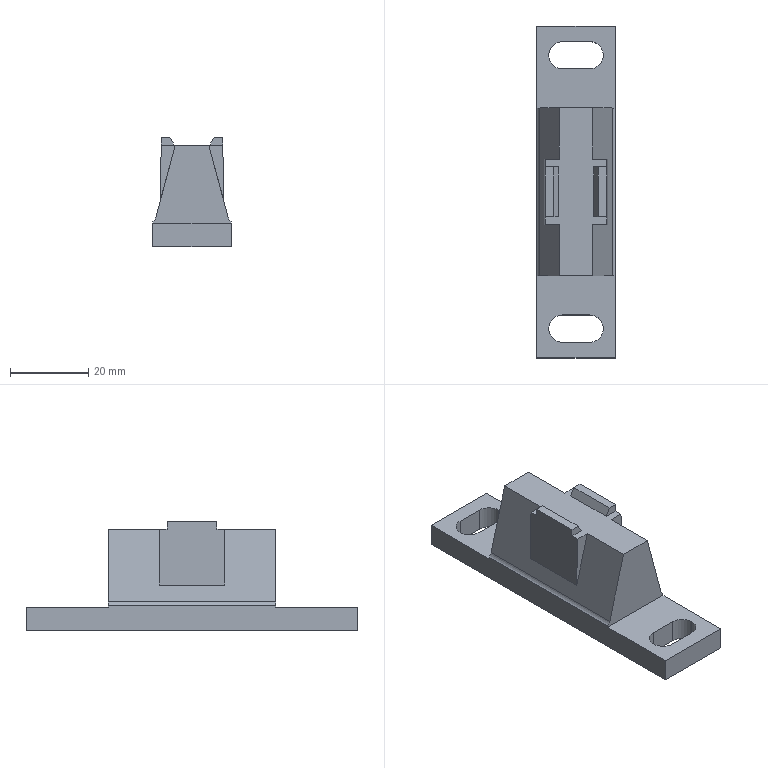Part | SolidWorks | features BaseBody 1 | 1 solid | 38 faces | box 20 x 85 x 28 mm | volume 22186 mm3 | plane 30 | cylinder 8 | commonest cylinder face diameters 7 x6 4 x2
STEP:
#1=CARTESIAN_POINT('',(7.,-35.,-41.));
#2=VERTEX_POINT('',#1);
#3=CARTESIAN_POINT('',(3.5,-31.5,-41.));
#4=VERTEX_POINT('',#3);
#5=CARTESIAN_POINT('',(3.5,-35.,-41.));
#6=DIRECTION('',(0.,0.,1.));
#7=DIRECTION('',(0.,-1.,0.));
#8=AXIS2_PLACEMENT_3D('',#5,#6,#7);
#9=CIRCLE('',#8,3.5);
#10=EDGE_CURVE('',#2,#4,#9,.T.);
#11=ORIENTED_EDGE('',*,*,#10,.F.);
#12=CARTESIAN_POINT('',(7.,-35.,-35.));
#13=VERTEX_POINT('',#12);
#14=CARTESIAN_POINT('',(7.,-35.,-41.));
#15=DIRECTION('',(0.,0.,1.));
#16=VECTOR('',#15,1000.);
#17=LINE('',#14,#16);
#18=EDGE_CURVE('',#2,#13,#17,.T.);
#19=ORIENTED_EDGE('',*,*,#18,.T.);
#20=CARTESIAN_POINT('',(3.5,-31.5,-35.));
#21=VERTEX_POINT('',#20);
#22=CARTESIAN_POINT('',(3.5,-35.,-35.));
#23=DIRECTION('',(0.,0.,1.));
#24=DIRECTION('',(0.,-1.,0.));
#25=AXIS2_PLACEMENT_3D('',#22,#23,#24);
#26=CIRCLE('',#25,3.5);
#27=EDGE_CURVE('',#13,#21,#26,.T.);
#28=ORIENTED_EDGE('',*,*,#27,.T.);
#29=CARTESIAN_POINT('',(3.5,-31.5,-41.));
#30=DIRECTION('',(0.,0.,1.));
#31=VECTOR('',#30,1000.);
#32=LINE('',#29,#31);
#33=EDGE_CURVE('',#4,#21,#32,.T.);
#34=ORIENTED_EDGE('',*,*,#33,.F.);
#35=EDGE_LOOP('',(#11,#19,#28,#34));
#36=FACE_OUTER_BOUND('',#35,.T.);
#37=CARTESIAN_POINT('',(3.5,-35.,-41.));
#38=DIRECTION('',(0.,0.,1.));
#39=DIRECTION('',(1.,0.,0.));
#40=AXIS2_PLACEMENT_3D('',#37,#38,#39);
#41=CYLINDRICAL_SURFACE('',#40,3.5);
#42=ADVANCED_FACE('',(#36),#41,.F.);
#43=CARTESIAN_POINT('',(7.,35.,-41.));
#44=VERTEX_POINT('',#43);
#45=CARTESIAN_POINT('',(3.5,38.5,-41.));
#46=VERTEX_POINT('',#45);
#47=CARTESIAN_POINT('',(3.5,35.,-41.));
#48=DIRECTION('',(0.,0.,1.));
#49=DIRECTION('',(0.,-1.,0.));
#50=AXIS2_PLACEMENT_3D('',#47,#48,#49);
#51=CIRCLE('',#50,3.5);
#52=EDGE_CURVE('',#44,#46,#51,.T.);
#53=ORIENTED_EDGE('',*,*,#52,.F.);
#54=CARTESIAN_POINT('',(7.,35.,-35.));
#55=VERTEX_POINT('',#54);
#56=CARTESIAN_POINT('',(7.,35.,-41.));
#57=DIRECTION('',(0.,0.,1.));
#58=VECTOR('',#57,1000.);
#59=LINE('',#56,#58);
#60=EDGE_CURVE('',#44,#55,#59,.T.);
#61=ORIENTED_EDGE('',*,*,#60,.T.);
#62=CARTESIAN_POINT('',(3.5,38.5,-35.));
#63=VERTEX_POINT('',#62);
#64=CARTESIAN_POINT('',(3.5,35.,-35.));
#65=DIRECTION('',(0.,0.,1.));
#66=DIRECTION('',(0.,-1.,0.));
#67=AXIS2_PLACEMENT_3D('',#64,#65,#66);
#68=CIRCLE('',#67,3.5);
#69=EDGE_CURVE('',#55,#63,#68,.T.);
#70=ORIENTED_EDGE('',*,*,#69,.T.);
#71=CARTESIAN_POINT('',(3.5,38.5,-41.));
#72=DIRECTION('',(0.,0.,1.));
#73=VECTOR('',#72,1000.);
#74=LINE('',#71,#73);
#75=EDGE_CURVE('',#46,#63,#74,.T.);
#76=ORIENTED_EDGE('',*,*,#75,.F.);
#77=EDGE_LOOP('',(#53,#61,#70,#76));
#78=FACE_OUTER_BOUND('',#77,.T.);
#79=CARTESIAN_POINT('',(3.5,35.,-41.));
#80=DIRECTION('',(0.,0.,1.));
#81=DIRECTION('',(1.,0.,0.));
#82=AXIS2_PLACEMENT_3D('',#79,#80,#81);
#83=CYLINDRICAL_SURFACE('',#82,3.5);
#84=ADVANCED_FACE('',(#78),#83,.F.);
#85=CARTESIAN_POINT('',(5.655,-6.4,-13.));
#86=VERTEX_POINT('',#85);
#87=CARTESIAN_POINT('',(4.5,-6.4,-15.));
#88=VERTEX_POINT('',#87);
#89=CARTESIAN_POINT('',(5.655,-6.4,-13.));
#90=DIRECTION('',(-0.5,0.,-0.866));
#91=VECTOR('',#90,1000.);
#92=LINE('',#89,#91);
#93=EDGE_CURVE('',#86,#88,#92,.T.);
#94=ORIENTED_EDGE('',*,*,#93,.F.);
#95=CARTESIAN_POINT('',(5.655,6.4,-13.));
#96=VERTEX_POINT('',#95);
#97=CARTESIAN_POINT('',(5.655,6.4,-13.));
#98=DIRECTION('',(0.,-1.,0.));
#99=VECTOR('',#98,1000.);
#100=LINE('',#97,#99);
#101=EDGE_CURVE('',#96,#86,#100,.T.);
#102=ORIENTED_EDGE('',*,*,#101,.F.);
#103=CARTESIAN_POINT('',(4.5,6.4,-15.));
#104=VERTEX_POINT('',#103);
#105=CARTESIAN_POINT('',(4.5,6.4,-15.));
#106=DIRECTION('',(0.5,0.,0.866));
#107=VECTOR('',#106,1000.);
#108=LINE('',#105,#107);
#109=EDGE_CURVE('',#104,#96,#108,.T.);
#110=ORIENTED_EDGE('',*,*,#109,.F.);
#111=CARTESIAN_POINT('',(4.5,6.4,-15.));
#112=DIRECTION('',(0.,-1.,0.));
#113=VECTOR('',#112,1000.);
#114=LINE('',#111,#113);
#115=EDGE_CURVE('',#104,#88,#114,.T.);
#116=ORIENTED_EDGE('',*,*,#115,.T.);
#117=EDGE_LOOP('',(#94,#102,#110,#116));
#118=FACE_OUTER_BOUND('',#117,.T.);
#119=CARTESIAN_POINT('',(4.5,8.4,-15.));
#120=DIRECTION('',(0.866,0.,-0.5));
#121=DIRECTION('',(-0.5,0.,-0.866));
#122=AXIS2_PLACEMENT_3D('',#119,#120,#121);
#123=PLANE('',#122);
#124=ADVANCED_FACE('',(#118),#123,.F.);
#125=ORIENTED_EDGE('',*,*,#93,.T.);
#126=CARTESIAN_POINT('',(7.885,-6.4,-15.));
#127=VERTEX_POINT('',#126);
#128=CARTESIAN_POINT('',(7.885,-6.4,-15.));
#129=DIRECTION('',(-1.,0.,0.));
#130=VECTOR('',#129,1000.);
#131=LINE('',#128,#130);
#132=EDGE_CURVE('',#127,#88,#131,.T.);
#133=ORIENTED_EDGE('',*,*,#132,.F.);
#134=CARTESIAN_POINT('',(7.85,-6.4,-13.));
#135=VERTEX_POINT('',#134);
#136=CARTESIAN_POINT('',(7.885,-6.4,-15.));
#137=DIRECTION('',(-0.01745,0.,0.9998));
#138=VECTOR('',#137,1000.);
#139=LINE('',#136,#138);
#140=EDGE_CURVE('',#127,#135,#139,.T.);
#141=ORIENTED_EDGE('',*,*,#140,.T.);
#142=CARTESIAN_POINT('',(7.85,-6.4,-13.));
#143=DIRECTION('',(-1.,0.,0.));
#144=VECTOR('',#143,1000.);
#145=LINE('',#142,#144);
#146=EDGE_CURVE('',#135,#86,#145,.T.);
#147=ORIENTED_EDGE('',*,*,#146,.T.);
#148=EDGE_LOOP('',(#125,#133,#141,#147));
#149=FACE_OUTER_BOUND('',#148,.T.);
#150=CARTESIAN_POINT('',(10.,-6.4,-15.));
#151=DIRECTION('',(0.,-1.,0.));
#152=DIRECTION('',(0.,0.,-1.));
#153=AXIS2_PLACEMENT_3D('',#150,#151,#152);
#154=PLANE('',#153);
#155=ADVANCED_FACE('',(#149),#154,.T.);
#156=ORIENTED_EDGE('',*,*,#146,.F.);
#157=CARTESIAN_POINT('',(7.85,6.4,-13.));
#158=VERTEX_POINT('',#157);
#159=CARTESIAN_POINT('',(7.85,6.4,-13.));
#160=DIRECTION('',(0.,-1.,0.));
#161=VECTOR('',#160,1000.);
#162=LINE('',#159,#161);
#163=EDGE_CURVE('',#158,#135,#162,.T.);
#164=ORIENTED_EDGE('',*,*,#163,.F.);
#165=CARTESIAN_POINT('',(5.655,6.4,-13.));
#166=DIRECTION('',(1.,0.,0.));
#167=VECTOR('',#166,1000.);
#168=LINE('',#165,#167);
#169=EDGE_CURVE('',#96,#158,#168,.T.);
#170=ORIENTED_EDGE('',*,*,#169,.F.);
#171=ORIENTED_EDGE('',*,*,#101,.T.);
#172=EDGE_LOOP('',(#156,#164,#170,#171));
#173=FACE_OUTER_BOUND('',#172,.T.);
#174=CARTESIAN_POINT('',(5.655,8.4,-13.));
#175=DIRECTION('',(0.,0.,-1.));
#176=DIRECTION('',(-1.,0.,0.));
#177=AXIS2_PLACEMENT_3D('',#174,#175,#176);
#178=PLANE('',#177);
#179=ADVANCED_FACE('',(#173),#178,.F.);
#180=ORIENTED_EDGE('',*,*,#109,.T.);
#181=ORIENTED_EDGE('',*,*,#169,.T.);
#182=CARTESIAN_POINT('',(7.885,6.4,-15.));
#183=VERTEX_POINT('',#182);
#184=CARTESIAN_POINT('',(7.85,6.4,-13.));
#185=DIRECTION('',(0.01745,0.,-0.9998));
#186=VECTOR('',#185,1000.);
#187=LINE('',#184,#186);
#188=EDGE_CURVE('',#158,#183,#187,.T.);
#189=ORIENTED_EDGE('',*,*,#188,.T.);
#190=CARTESIAN_POINT('',(7.885,6.4,-15.));
#191=DIRECTION('',(-1.,0.,0.));
#192=VECTOR('',#191,1000.);
#193=LINE('',#190,#192);
#194=EDGE_CURVE('',#183,#104,#193,.T.);
#195=ORIENTED_EDGE('',*,*,#194,.T.);
#196=EDGE_LOOP('',(#180,#181,#189,#195));
#197=FACE_OUTER_BOUND('',#196,.T.);
#198=CARTESIAN_POINT('',(10.,6.4,-12.));
#199=DIRECTION('',(0.,1.,0.));
#200=DIRECTION('',(0.,0.,1.));
#201=AXIS2_PLACEMENT_3D('',#198,#199,#200);
#202=PLANE('',#201);
#203=ADVANCED_FACE('',(#197),#202,.T.);
#204=CARTESIAN_POINT('',(4.3,8.4,-15.));
#205=VERTEX_POINT('',#204);
#206=CARTESIAN_POINT('',(7.885,8.4,-15.));
#207=VERTEX_POINT('',#206);
#208=CARTESIAN_POINT('',(4.3,8.4,-15.));
#209=DIRECTION('',(1.,0.,0.));
#210=VECTOR('',#209,1000.);
#211=LINE('',#208,#210);
#212=EDGE_CURVE('',#205,#207,#211,.T.);
#213=ORIENTED_EDGE('',*,*,#212,.F.);
#214=CARTESIAN_POINT('',(4.3,21.5,-15.));
#215=VERTEX_POINT('',#214);
#216=CARTESIAN_POINT('',(4.3,21.5,-15.));
#217=DIRECTION('',(0.,-1.,0.));
#218=VECTOR('',#217,1000.);
#219=LINE('',#216,#218);
#220=EDGE_CURVE('',#215,#205,#219,.T.);
#221=ORIENTED_EDGE('',*,*,#220,.F.);
#222=CARTESIAN_POINT('',(-4.3,21.5,-15.));
#223=VERTEX_POINT('',#222);
#224=CARTESIAN_POINT('',(-4.3,21.5,-15.));
#225=DIRECTION('',(1.,0.,0.));
#226=VECTOR('',#225,1000.);
#227=LINE('',#224,#226);
#228=EDGE_CURVE('',#223,#215,#227,.T.);
#229=ORIENTED_EDGE('',*,*,#228,.F.);
#230=CARTESIAN_POINT('',(-4.3,8.4,-15.));
#231=VERTEX_POINT('',#230);
#232=CARTESIAN_POINT('',(-4.3,21.5,-15.));
#233=DIRECTION('',(0.,-1.,0.));
#234=VECTOR('',#233,1000.);
#235=LINE('',#232,#234);
#236=EDGE_CURVE('',#223,#231,#235,.T.);
#237=ORIENTED_EDGE('',*,*,#236,.T.);
#238=CARTESIAN_POINT('',(-7.885,8.4,-15.));
#239=VERTEX_POINT('',#238);
#240=CARTESIAN_POINT('',(-7.885,8.4,-15.));
#241=DIRECTION('',(1.,0.,0.));
#242=VECTOR('',#241,1000.);
#243=LINE('',#240,#242);
#244=EDGE_CURVE('',#239,#231,#243,.T.);
#245=ORIENTED_EDGE('',*,*,#244,.F.);
#246=CARTESIAN_POINT('',(-7.885,6.4,-15.));
#247=VERTEX_POINT('',#246);
#248=CARTESIAN_POINT('',(-7.885,8.4,-15.));
#249=DIRECTION('',(0.,-1.,0.));
#250=VECTOR('',#249,1000.);
#251=LINE('',#248,#250);
#252=EDGE_CURVE('',#239,#247,#251,.T.);
#253=ORIENTED_EDGE('',*,*,#252,.T.);
#254=CARTESIAN_POINT('',(-4.5,6.4,-15.));
#255=VERTEX_POINT('',#254);
#256=CARTESIAN_POINT('',(-4.5,6.4,-15.));
#257=DIRECTION('',(-1.,0.,0.));
#258=VECTOR('',#257,1000.);
#259=LINE('',#256,#258);
#260=EDGE_CURVE('',#255,#247,#259,.T.);
#261=ORIENTED_EDGE('',*,*,#260,.F.);
#262=CARTESIAN_POINT('',(-4.5,-6.4,-15.));
#263=VERTEX_POINT('',#262);
#264=CARTESIAN_POINT('',(-4.5,6.4,-15.));
#265=DIRECTION('',(0.,-1.,0.));
#266=VECTOR('',#265,1000.);
#267=LINE('',#264,#266);
#268=EDGE_CURVE('',#255,#263,#267,.T.);
#269=ORIENTED_EDGE('',*,*,#268,.T.);
#270=CARTESIAN_POINT('',(-7.885,-6.4,-15.));
#271=VERTEX_POINT('',#270);
#272=CARTESIAN_POINT('',(-4.5,-6.4,-15.));
#273=DIRECTION('',(-1.,0.,0.));
#274=VECTOR('',#273,1000.);
#275=LINE('',#272,#274);
#276=EDGE_CURVE('',#263,#271,#275,.T.);
#277=ORIENTED_EDGE('',*,*,#276,.T.);
#278=CARTESIAN_POINT('',(-7.885,-8.4,-15.));
#279=VERTEX_POINT('',#278);
#280=CARTESIAN_POINT('',(-7.885,-6.4,-15.));
#281=DIRECTION('',(0.,-1.,0.));
#282=VECTOR('',#281,1000.);
#283=LINE('',#280,#282);
#284=EDGE_CURVE('',#271,#279,#283,.T.);
#285=ORIENTED_EDGE('',*,*,#284,.T.);
#286=CARTESIAN_POINT('',(-4.3,-8.4,-15.));
#287=VERTEX_POINT('',#286);
#288=CARTESIAN_POINT('',(-7.885,-8.4,-15.));
#289=DIRECTION('',(1.,0.,0.));
#290=VECTOR('',#289,1000.);
#291=LINE('',#288,#290);
#292=EDGE_CURVE('',#279,#287,#291,.T.);
#293=ORIENTED_EDGE('',*,*,#292,.T.);
#294=CARTESIAN_POINT('',(-4.3,-21.5,-15.));
#295=VERTEX_POINT('',#294);
#296=CARTESIAN_POINT('',(-4.3,-8.4,-15.));
#297=DIRECTION('',(0.,-1.,0.));
#298=VECTOR('',#297,1000.);
#299=LINE('',#296,#298);
#300=EDGE_CURVE('',#287,#295,#299,.T.);
#301=ORIENTED_EDGE('',*,*,#300,.T.);
#302=CARTESIAN_POINT('',(4.3,-21.5,-15.));
#303=VERTEX_POINT('',#302);
#304=CARTESIAN_POINT('',(-4.3,-21.5,-15.));
#305=DIRECTION('',(1.,0.,0.));
#306=VECTOR('',#305,1000.);
#307=LINE('',#304,#306);
#308=EDGE_CURVE('',#295,#303,#307,.T.);
#309=ORIENTED_EDGE('',*,*,#308,.T.);
#310=CARTESIAN_POINT('',(4.3,-8.4,-15.));
#311=VERTEX_POINT('',#310);
#312=CARTESIAN_POINT('',(4.3,-8.4,-15.));
#313=DIRECTION('',(0.,-1.,0.));
#314=VECTOR('',#313,1000.);
#315=LINE('',#312,#314);
#316=EDGE_CURVE('',#311,#303,#315,.T.);
#317=ORIENTED_EDGE('',*,*,#316,.F.);
#318=CARTESIAN_POINT('',(7.885,-8.4,-15.));
#319=VERTEX_POINT('',#318);
#320=CARTESIAN_POINT('',(4.3,-8.4,-15.));
#321=DIRECTION('',(1.,0.,0.));
#322=VECTOR('',#321,1000.);
#323=LINE('',#320,#322);
#324=EDGE_CURVE('',#311,#319,#323,.T.);
#325=ORIENTED_EDGE('',*,*,#324,.T.);
#326=CARTESIAN_POINT('',(7.885,-8.4,-15.));
#327=DIRECTION('',(0.,1.,0.));
#328=VECTOR('',#327,1000.);
#329=LINE('',#326,#328);
#330=EDGE_CURVE('',#319,#127,#329,.T.);
#331=ORIENTED_EDGE('',*,*,#330,.T.);
#332=ORIENTED_EDGE('',*,*,#132,.T.);
#333=ORIENTED_EDGE('',*,*,#115,.F.);
#334=ORIENTED_EDGE('',*,*,#194,.F.);
#335=CARTESIAN_POINT('',(7.885,6.4,-15.));
#336=DIRECTION('',(0.,1.,0.));
#337=VECTOR('',#336,1000.);
#338=LINE('',#335,#337);
#339=EDGE_CURVE('',#183,#207,#338,.T.);
#340=ORIENTED_EDGE('',*,*,#339,.T.);
#341=EDGE_LOOP('',(#213,#221,#229,#237,#245,#253,#261,#269,#277,#285,#293,#301,#309,#317,#325,#331,#332,#333,#334,#340));
#342=FACE_OUTER_BOUND('',#341,.T.);
#343=CARTESIAN_POINT('',(-4.3,21.5,-15.));
#344=DIRECTION('',(0.,0.,-1.));
#345=DIRECTION('',(-1.,0.,0.));
#346=AXIS2_PLACEMENT_3D('',#343,#344,#345);
#347=PLANE('',#346);
#348=ADVANCED_FACE('',(#342),#347,.F.);
#349=ORIENTED_EDGE('',*,*,#330,.F.);
#350=CARTESIAN_POINT('',(8.135,-8.4,-29.311));
#351=VERTEX_POINT('',#350);
#352=CARTESIAN_POINT('',(7.885,-8.4,-15.));
#353=DIRECTION('',(0.01745,0.,-0.9998));
#354=VECTOR('',#353,1000.);
#355=LINE('',#352,#354);
#356=EDGE_CURVE('',#319,#351,#355,.T.);
#357=ORIENTED_EDGE('',*,*,#356,.T.);
#358=CARTESIAN_POINT('',(8.135,8.4,-29.311));
#359=VERTEX_POINT('',#358);
#360=CARTESIAN_POINT('',(8.135,-8.4,-29.311));
#361=DIRECTION('',(0.,1.,0.));
#362=VECTOR('',#361,1000.);
#363=LINE('',#360,#362);
#364=EDGE_CURVE('',#351,#359,#363,.T.);
#365=ORIENTED_EDGE('',*,*,#364,.T.);
#366=CARTESIAN_POINT('',(7.885,8.4,-15.));
#367=DIRECTION('',(0.01745,0.,-0.9998));
#368=VECTOR('',#367,1000.);
#369=LINE('',#366,#368);
#370=EDGE_CURVE('',#207,#359,#369,.T.);
#371=ORIENTED_EDGE('',*,*,#370,.F.);
#372=ORIENTED_EDGE('',*,*,#339,.F.);
#373=ORIENTED_EDGE('',*,*,#188,.F.);
#374=ORIENTED_EDGE('',*,*,#163,.T.);
#375=ORIENTED_EDGE('',*,*,#140,.F.);
#376=EDGE_LOOP('',(#349,#357,#365,#371,#372,#373,#374,#375));
#377=FACE_OUTER_BOUND('',#376,.T.);
#378=CARTESIAN_POINT('',(7.85,8.4,-13.));
#379=DIRECTION('',(-0.9998,0.,-0.01745));
#380=DIRECTION('',(-0.01745,0.,0.9998));
#381=AXIS2_PLACEMENT_3D('',#378,#379,#380);
#382=PLANE('',#381);
#383=ADVANCED_FACE('',(#377),#382,.F.);
#384=ORIENTED_EDGE('',*,*,#212,.T.);
#385=ORIENTED_EDGE('',*,*,#370,.T.);
#386=CARTESIAN_POINT('',(4.3,8.4,-15.));
#387=DIRECTION('',(0.2588,0.,-0.9659));
#388=VECTOR('',#387,1000.);
#389=LINE('',#386,#388);
#390=EDGE_CURVE('',#205,#359,#389,.T.);
#391=ORIENTED_EDGE('',*,*,#390,.F.);
#392=EDGE_LOOP('',(#384,#385,#391));
#393=FACE_OUTER_BOUND('',#392,.T.);
#394=CARTESIAN_POINT('',(0.,8.4,0.));
#395=DIRECTION('',(0.,1.,0.));
#396=DIRECTION('',(0.,0.,1.));
#397=AXIS2_PLACEMENT_3D('',#394,#395,#396);
#398=PLANE('',#397);
#399=ADVANCED_FACE('',(#393),#398,.T.);
#400=ORIENTED_EDGE('',*,*,#220,.T.);
#401=ORIENTED_EDGE('',*,*,#390,.T.);
#402=ORIENTED_EDGE('',*,*,#364,.F.);
#403=CARTESIAN_POINT('',(4.3,-8.4,-15.));
#404=DIRECTION('',(0.2588,0.,-0.9659));
#405=VECTOR('',#404,1000.);
#406=LINE('',#403,#405);
#407=EDGE_CURVE('',#311,#351,#406,.T.);
#408=ORIENTED_EDGE('',*,*,#407,.F.);
#409=ORIENTED_EDGE('',*,*,#316,.T.);
#410=CARTESIAN_POINT('',(9.262,-21.5,-33.518));
#411=VERTEX_POINT('',#410);
#412=CARTESIAN_POINT('',(4.3,-21.5,-15.));
#413=DIRECTION('',(0.2588,0.,-0.9659));
#414=VECTOR('',#413,1000.);
#415=LINE('',#412,#414);
#416=EDGE_CURVE('',#303,#411,#415,.T.);
#417=ORIENTED_EDGE('',*,*,#416,.T.);
#418=CARTESIAN_POINT('',(9.262,21.5,-33.518));
#419=VERTEX_POINT('',#418);
#420=CARTESIAN_POINT('',(9.262,21.5,-33.518));
#421=DIRECTION('',(0.,-1.,0.));
#422=VECTOR('',#421,1000.);
#423=LINE('',#420,#422);
#424=EDGE_CURVE('',#419,#411,#423,.T.);
#425=ORIENTED_EDGE('',*,*,#424,.F.);
#426=CARTESIAN_POINT('',(4.3,21.5,-15.));
#427=DIRECTION('',(0.2588,0.,-0.9659));
#428=VECTOR('',#427,1000.);
#429=LINE('',#426,#428);
#430=EDGE_CURVE('',#215,#419,#429,.T.);
#431=ORIENTED_EDGE('',*,*,#430,.F.);
#432=EDGE_LOOP('',(#400,#401,#402,#408,#409,#417,#425,#431));
#433=FACE_OUTER_BOUND('',#432,.T.);
#434=CARTESIAN_POINT('',(4.3,21.5,-15.));
#435=DIRECTION('',(-0.9659,0.,-0.2588));
#436=DIRECTION('',(-0.2588,0.,0.9659));
#437=AXIS2_PLACEMENT_3D('',#434,#435,#436);
#438=PLANE('',#437);
#439=ADVANCED_FACE('',(#433),#438,.F.);
#440=CARTESIAN_POINT('',(-10.,21.5,-35.));
#441=VERTEX_POINT('',#440);
#442=CARTESIAN_POINT('',(-10.,21.5,-34.605));
#443=VERTEX_POINT('',#442);
#444=CARTESIAN_POINT('',(-10.,21.5,-35.));
#445=DIRECTION('',(0.,0.,1.));
#446=VECTOR('',#445,1000.);
#447=LINE('',#444,#446);
#448=EDGE_CURVE('',#441,#443,#447,.T.);
#449=ORIENTED_EDGE('',*,*,#448,.T.);
#450=CARTESIAN_POINT('',(-9.262,21.5,-33.518));
#451=VERTEX_POINT('',#450);
#452=CARTESIAN_POINT('',(-11.194,21.5,-33.));
#453=DIRECTION('',(0.,1.,0.));
#454=DIRECTION('',(0.9659,0.,-0.2588));
#455=AXIS2_PLACEMENT_3D('',#452,#453,#454);
#456=CIRCLE('',#455,2.);
#457=EDGE_CURVE('',#451,#443,#456,.T.);
#458=ORIENTED_EDGE('',*,*,#457,.F.);
#459=CARTESIAN_POINT('',(-9.262,21.5,-33.518));
#460=DIRECTION('',(0.2588,0.,0.9659));
#461=VECTOR('',#460,1000.);
#462=LINE('',#459,#461);
#463=EDGE_CURVE('',#451,#223,#462,.T.);
#464=ORIENTED_EDGE('',*,*,#463,.T.);
#465=ORIENTED_EDGE('',*,*,#228,.T.);
#466=ORIENTED_EDGE('',*,*,#430,.T.);
#467=CARTESIAN_POINT('',(10.,21.5,-34.605));
#468=VERTEX_POINT('',#467);
#469=CARTESIAN_POINT('',(11.194,21.5,-33.));
#470=DIRECTION('',(0.,1.,0.));
#471=DIRECTION('',(-0.5968,0.,-0.8024));
#472=AXIS2_PLACEMENT_3D('',#469,#470,#471);
#473=CIRCLE('',#472,2.);
#474=EDGE_CURVE('',#468,#419,#473,.T.);
#475=ORIENTED_EDGE('',*,*,#474,.F.);
#476=CARTESIAN_POINT('',(10.,21.5,-35.));
#477=VERTEX_POINT('',#476);
#478=CARTESIAN_POINT('',(10.,21.5,-34.605));
#479=DIRECTION('',(0.,0.,-1.));
#480=VECTOR('',#479,1000.);
#481=LINE('',#478,#480);
#482=EDGE_CURVE('',#468,#477,#481,.T.);
#483=ORIENTED_EDGE('',*,*,#482,.T.);
#484=CARTESIAN_POINT('',(10.,21.5,-35.));
#485=DIRECTION('',(-1.,0.,0.));
#486=VECTOR('',#485,1000.);
#487=LINE('',#484,#486);
#488=EDGE_CURVE('',#477,#441,#487,.T.);
#489=ORIENTED_EDGE('',*,*,#488,.T.);
#490=EDGE_LOOP('',(#449,#458,#464,#465,#466,#475,#483,#489));
#491=FACE_OUTER_BOUND('',#490,.T.);
#492=CARTESIAN_POINT('',(-11.194,21.5,-33.));
#493=DIRECTION('',(0.,1.,0.));
#494=DIRECTION('',(0.,0.,1.));
#495=AXIS2_PLACEMENT_3D('',#492,#493,#494);
#496=PLANE('',#495);
#497=ADVANCED_FACE('',(#491),#496,.T.);
#498=CARTESIAN_POINT('',(-8.135,8.4,-29.311));
#499=VERTEX_POINT('',#498);
#500=CARTESIAN_POINT('',(-8.135,-8.4,-29.311));
#501=VERTEX_POINT('',#500);
#502=CARTESIAN_POINT('',(-8.135,8.4,-29.311));
#503=DIRECTION('',(0.,-1.,0.));
#504=VECTOR('',#503,1000.);
#505=LINE('',#502,#504);
#506=EDGE_CURVE('',#499,#501,#505,.T.);
#507=ORIENTED_EDGE('',*,*,#506,.F.);
#508=CARTESIAN_POINT('',(-8.135,8.4,-29.311));
#509=DIRECTION('',(0.2588,0.,0.9659));
#510=VECTOR('',#509,1000.);
#511=LINE('',#508,#510);
#512=EDGE_CURVE('',#499,#231,#511,.T.);
#513=ORIENTED_EDGE('',*,*,#512,.T.);
#514=ORIENTED_EDGE('',*,*,#236,.F.);
#515=ORIENTED_EDGE('',*,*,#463,.F.);
#516=CARTESIAN_POINT('',(-9.262,-21.5,-33.518));
#517=VERTEX_POINT('',#516);
#518=CARTESIAN_POINT('',(-9.262,21.5,-33.518));
#519=DIRECTION('',(0.,-1.,0.));
#520=VECTOR('',#519,1000.);
#521=LINE('',#518,#520);
#522=EDGE_CURVE('',#451,#517,#521,.T.);
#523=ORIENTED_EDGE('',*,*,#522,.T.);
#524=CARTESIAN_POINT('',(-9.262,-21.5,-33.518));
#525=DIRECTION('',(0.2588,0.,0.9659));
#526=VECTOR('',#525,1000.);
#527=LINE('',#524,#526);
#528=EDGE_CURVE('',#517,#295,#527,.T.);
#529=ORIENTED_EDGE('',*,*,#528,.T.);
#530=ORIENTED_EDGE('',*,*,#300,.F.);
#531=CARTESIAN_POINT('',(-8.135,-8.4,-29.311));
#532=DIRECTION('',(0.2588,0.,0.9659));
#533=VECTOR('',#532,1000.);
#534=LINE('',#531,#533);
#535=EDGE_CURVE('',#501,#287,#534,.T.);
#536=ORIENTED_EDGE('',*,*,#535,.F.);
#537=EDGE_LOOP('',(#507,#513,#514,#515,#523,#529,#530,#536));
#538=FACE_OUTER_BOUND('',#537,.T.);
#539=CARTESIAN_POINT('',(-9.262,21.5,-33.518));
#540=DIRECTION('',(0.9659,0.,-0.2588));
#541=DIRECTION('',(-0.2588,0.,-0.9659));
#542=AXIS2_PLACEMENT_3D('',#539,#540,#541);
#543=PLANE('',#542);
#544=ADVANCED_FACE('',(#538),#543,.F.);
#545=CARTESIAN_POINT('',(-8.135,8.4,-29.311));
#546=DIRECTION('',(0.01745,0.,0.9998));
#547=VECTOR('',#546,1000.);
#548=LINE('',#545,#547);
#549=EDGE_CURVE('',#499,#239,#548,.T.);
#550=ORIENTED_EDGE('',*,*,#549,.T.);
#551=ORIENTED_EDGE('',*,*,#244,.T.);
#552=ORIENTED_EDGE('',*,*,#512,.F.);
#553=EDGE_LOOP('',(#550,#551,#552));
#554=FACE_OUTER_BOUND('',#553,.T.);
#555=CARTESIAN_POINT('',(0.,8.4,0.));
#556=DIRECTION('',(0.,1.,0.));
#557=DIRECTION('',(0.,0.,1.));
#558=AXIS2_PLACEMENT_3D('',#555,#556,#557);
#559=PLANE('',#558);
#560=ADVANCED_FACE('',(#554),#559,.T.);
#561=ORIENTED_EDGE('',*,*,#284,.F.);
#562=CARTESIAN_POINT('',(-7.85,-6.4,-13.));
#563=VERTEX_POINT('',#562);
#564=CARTESIAN_POINT('',(-7.85,-6.4,-13.));
#565=DIRECTION('',(-0.01745,0.,-0.9998));
#566=VECTOR('',#565,1000.);
#567=LINE('',#564,#566);
#568=EDGE_CURVE('',#563,#271,#567,.T.);
#569=ORIENTED_EDGE('',*,*,#568,.F.);
#570=CARTESIAN_POINT('',(-7.85,6.4,-13.));
#571=VERTEX_POINT('',#570);
#572=CARTESIAN_POINT('',(-7.85,6.4,-13.));
#573=DIRECTION('',(0.,-1.,0.));
#574=VECTOR('',#573,1000.);
#575=LINE('',#572,#574);
#576=EDGE_CURVE('',#571,#563,#575,.T.);
#577=ORIENTED_EDGE('',*,*,#576,.F.);
#578=CARTESIAN_POINT('',(-7.885,6.4,-15.));
#579=DIRECTION('',(0.01745,0.,0.9998));
#580=VECTOR('',#579,1000.);
#581=LINE('',#578,#580);
#582=EDGE_CURVE('',#247,#571,#581,.T.);
#583=ORIENTED_EDGE('',*,*,#582,.F.);
#584=ORIENTED_EDGE('',*,*,#252,.F.);
#585=ORIENTED_EDGE('',*,*,#549,.F.);
#586=ORIENTED_EDGE('',*,*,#506,.T.);
#587=CARTESIAN_POINT('',(-8.135,-8.4,-29.311));
#588=DIRECTION('',(0.01745,0.,0.9998));
#589=VECTOR('',#588,1000.);
#590=LINE('',#587,#589);
#591=EDGE_CURVE('',#501,#279,#590,.T.);
#592=ORIENTED_EDGE('',*,*,#591,.T.);
#593=EDGE_LOOP('',(#561,#569,#577,#583,#584,#585,#586,#592));
#594=FACE_OUTER_BOUND('',#593,.T.);
#595=CARTESIAN_POINT('',(-8.234,8.4,-35.));
#596=DIRECTION('',(0.9998,0.,-0.01745));
#597=DIRECTION('',(-0.01745,0.,-0.9998));
#598=AXIS2_PLACEMENT_3D('',#595,#596,#597);
#599=PLANE('',#598);
#600=ADVANCED_FACE('',(#594),#599,.F.);
#601=ORIENTED_EDGE('',*,*,#582,.T.);
#602=CARTESIAN_POINT('',(-5.655,6.4,-13.));
#603=VERTEX_POINT('',#602);
#604=CARTESIAN_POINT('',(-7.85,6.4,-13.));
#605=DIRECTION('',(1.,0.,0.));
#606=VECTOR('',#605,1000.);
#607=LINE('',#604,#606);
#608=EDGE_CURVE('',#571,#603,#607,.T.);
#609=ORIENTED_EDGE('',*,*,#608,.T.);
#610=CARTESIAN_POINT('',(-5.655,6.4,-13.));
#611=DIRECTION('',(0.5,0.,-0.866));
#612=VECTOR('',#611,1000.);
#613=LINE('',#610,#612);
#614=EDGE_CURVE('',#603,#255,#613,.T.);
#615=ORIENTED_EDGE('',*,*,#614,.T.);
#616=ORIENTED_EDGE('',*,*,#260,.T.);
#617=EDGE_LOOP('',(#601,#609,#615,#616));
#618=FACE_OUTER_BOUND('',#617,.T.);
#619=CARTESIAN_POINT('',(10.,6.4,-12.));
#620=DIRECTION('',(0.,1.,0.));
#621=DIRECTION('',(0.,0.,1.));
#622=AXIS2_PLACEMENT_3D('',#619,#620,#621);
#623=PLANE('',#622);
#624=ADVANCED_FACE('',(#618),#623,.T.);
#625=CARTESIAN_POINT('',(-5.655,-6.4,-13.));
#626=VERTEX_POINT('',#625);
#627=CARTESIAN_POINT('',(-4.5,-6.4,-15.));
#628=DIRECTION('',(-0.5,0.,0.866));
#629=VECTOR('',#628,1000.);
#630=LINE('',#627,#629);
#631=EDGE_CURVE('',#263,#626,#630,.T.);
#632=ORIENTED_EDGE('',*,*,#631,.F.);
#633=ORIENTED_EDGE('',*,*,#268,.F.);
#634=ORIENTED_EDGE('',*,*,#614,.F.);
#635=CARTESIAN_POINT('',(-5.655,6.4,-13.));
#636=DIRECTION('',(0.,-1.,0.));
#637=VECTOR('',#636,1000.);
#638=LINE('',#635,#637);
#639=EDGE_CURVE('',#603,#626,#638,.T.);
#640=ORIENTED_EDGE('',*,*,#639,.T.);
#641=EDGE_LOOP('',(#632,#633,#634,#640));
#642=FACE_OUTER_BOUND('',#641,.T.);
#643=CARTESIAN_POINT('',(-5.655,8.4,-13.));
#644=DIRECTION('',(-0.866,0.,-0.5));
#645=DIRECTION('',(-0.5,0.,0.866));
#646=AXIS2_PLACEMENT_3D('',#643,#644,#645);
#647=PLANE('',#646);
#648=ADVANCED_FACE('',(#642),#647,.F.);
#649=ORIENTED_EDGE('',*,*,#568,.T.);
#650=ORIENTED_EDGE('',*,*,#276,.F.);
#651=ORIENTED_EDGE('',*,*,#631,.T.);
#652=CARTESIAN_POINT('',(-5.655,-6.4,-13.));
#653=DIRECTION('',(-1.,0.,0.));
#654=VECTOR('',#653,1000.);
#655=LINE('',#652,#654);
#656=EDGE_CURVE('',#626,#563,#655,.T.);
#657=ORIENTED_EDGE('',*,*,#656,.T.);
#658=EDGE_LOOP('',(#649,#650,#651,#657));
#659=FACE_OUTER_BOUND('',#658,.T.);
#660=CARTESIAN_POINT('',(10.,-6.4,-15.));
#661=DIRECTION('',(0.,-1.,0.));
#662=DIRECTION('',(0.,0.,-1.));
#663=AXIS2_PLACEMENT_3D('',#660,#661,#662);
#664=PLANE('',#663);
#665=ADVANCED_FACE('',(#659),#664,.T.);
#666=ORIENTED_EDGE('',*,*,#292,.F.);
#667=ORIENTED_EDGE('',*,*,#591,.F.);
#668=ORIENTED_EDGE('',*,*,#535,.T.);
#669=EDGE_LOOP('',(#666,#667,#668));
#670=FACE_OUTER_BOUND('',#669,.T.);
#671=CARTESIAN_POINT('',(0.,-8.4,0.));
#672=DIRECTION('',(0.,1.,0.));
#673=DIRECTION('',(0.,0.,1.));
#674=AXIS2_PLACEMENT_3D('',#671,#672,#673);
#675=PLANE('',#674);
#676=ADVANCED_FACE('',(#670),#675,.F.);
#677=CARTESIAN_POINT('',(-10.,-21.5,-35.));
#678=VERTEX_POINT('',#677);
#679=CARTESIAN_POINT('',(-10.,-21.5,-34.605));
#680=VERTEX_POINT('',#679);
#681=CARTESIAN_POINT('',(-10.,-21.5,-35.));
#682=DIRECTION('',(0.,0.,1.));
#683=VECTOR('',#682,1000.);
#684=LINE('',#681,#683);
#685=EDGE_CURVE('',#678,#680,#684,.T.);
#686=ORIENTED_EDGE('',*,*,#685,.F.);
#687=CARTESIAN_POINT('',(10.,-21.5,-35.));
#688=VERTEX_POINT('',#687);
#689=CARTESIAN_POINT('',(10.,-21.5,-35.));
#690=DIRECTION('',(-1.,0.,0.));
#691=VECTOR('',#690,1000.);
#692=LINE('',#689,#691);
#693=EDGE_CURVE('',#688,#678,#692,.T.);
#694=ORIENTED_EDGE('',*,*,#693,.F.);
#695=CARTESIAN_POINT('',(10.,-21.5,-34.605));
#696=VERTEX_POINT('',#695);
#697=CARTESIAN_POINT('',(10.,-21.5,-34.605));
#698=DIRECTION('',(0.,0.,-1.));
#699=VECTOR('',#698,1000.);
#700=LINE('',#697,#699);
#701=EDGE_CURVE('',#696,#688,#700,.T.);
#702=ORIENTED_EDGE('',*,*,#701,.F.);
#703=CARTESIAN_POINT('',(11.194,-21.5,-33.));
#704=DIRECTION('',(0.,1.,0.));
#705=DIRECTION('',(-0.5968,0.,-0.8024));
#706=AXIS2_PLACEMENT_3D('',#703,#704,#705);
#707=CIRCLE('',#706,2.);
#708=EDGE_CURVE('',#696,#411,#707,.T.);
#709=ORIENTED_EDGE('',*,*,#708,.T.);
#710=ORIENTED_EDGE('',*,*,#416,.F.);
#711=ORIENTED_EDGE('',*,*,#308,.F.);
#712=ORIENTED_EDGE('',*,*,#528,.F.);
#713=CARTESIAN_POINT('',(-11.194,-21.5,-33.));
#714=DIRECTION('',(0.,1.,0.));
#715=DIRECTION('',(0.9659,0.,-0.2588));
#716=AXIS2_PLACEMENT_3D('',#713,#714,#715);
#717=CIRCLE('',#716,2.);
#718=EDGE_CURVE('',#517,#680,#717,.T.);
#719=ORIENTED_EDGE('',*,*,#718,.T.);
#720=EDGE_LOOP('',(#686,#694,#702,#709,#710,#711,#712,#719));
#721=FACE_OUTER_BOUND('',#720,.T.);
#722=CARTESIAN_POINT('',(-11.194,-21.5,-33.));
#723=DIRECTION('',(0.,1.,0.));
#724=DIRECTION('',(0.,0.,1.));
#725=AXIS2_PLACEMENT_3D('',#722,#723,#724);
#726=PLANE('',#725);
#727=ADVANCED_FACE('',(#721),#726,.F.);
#728=ORIENTED_EDGE('',*,*,#356,.F.);
#729=ORIENTED_EDGE('',*,*,#324,.F.);
#730=ORIENTED_EDGE('',*,*,#407,.T.);
#731=EDGE_LOOP('',(#728,#729,#730));
#732=FACE_OUTER_BOUND('',#731,.T.);
#733=CARTESIAN_POINT('',(0.,-8.4,0.));
#734=DIRECTION('',(0.,1.,0.));
#735=DIRECTION('',(0.,0.,1.));
#736=AXIS2_PLACEMENT_3D('',#733,#734,#735);
#737=PLANE('',#736);
#738=ADVANCED_FACE('',(#732),#737,.F.);
#739=ORIENTED_EDGE('',*,*,#708,.F.);
#740=CARTESIAN_POINT('',(10.,21.5,-34.605));
#741=DIRECTION('',(0.,-1.,0.));
#742=VECTOR('',#741,1000.);
#743=LINE('',#740,#742);
#744=EDGE_CURVE('',#468,#696,#743,.T.);
#745=ORIENTED_EDGE('',*,*,#744,.F.);
#746=ORIENTED_EDGE('',*,*,#474,.T.);
#747=ORIENTED_EDGE('',*,*,#424,.T.);
#748=EDGE_LOOP('',(#739,#745,#746,#747));
#749=FACE_OUTER_BOUND('',#748,.T.);
#750=CARTESIAN_POINT('',(11.194,21.5,-33.));
#751=DIRECTION('',(0.,-1.,0.));
#752=DIRECTION('',(0.,0.,-1.));
#753=AXIS2_PLACEMENT_3D('',#750,#751,#752);
#754=CYLINDRICAL_SURFACE('',#753,2.);
#755=ADVANCED_FACE('',(#749),#754,.F.);
#756=CARTESIAN_POINT('',(-10.,42.5,-35.));
#757=VERTEX_POINT('',#756);
#758=CARTESIAN_POINT('',(-10.,42.5,-35.));
#759=DIRECTION('',(0.,-1.,0.));
#760=VECTOR('',#759,1000.);
#761=LINE('',#758,#760);
#762=EDGE_CURVE('',#757,#441,#761,.T.);
#763=ORIENTED_EDGE('',*,*,#762,.F.);
#764=CARTESIAN_POINT('',(-10.,42.5,-41.));
#765=VERTEX_POINT('',#764);
#766=CARTESIAN_POINT('',(-10.,42.5,-41.));
#767=DIRECTION('',(0.,0.,1.));
#768=VECTOR('',#767,1000.);
#769=LINE('',#766,#768);
#770=EDGE_CURVE('',#765,#757,#769,.T.);
#771=ORIENTED_EDGE('',*,*,#770,.F.);
#772=CARTESIAN_POINT('',(-10.,-42.5,-41.));
#773=VERTEX_POINT('',#772);
#774=CARTESIAN_POINT('',(-10.,42.5,-41.));
#775=DIRECTION('',(0.,-1.,0.));
#776=VECTOR('',#775,1000.);
#777=LINE('',#774,#776);
#778=EDGE_CURVE('',#765,#773,#777,.T.);
#779=ORIENTED_EDGE('',*,*,#778,.T.);
#780=CARTESIAN_POINT('',(-10.,-42.5,-35.));
#781=VERTEX_POINT('',#780);
#782=CARTESIAN_POINT('',(-10.,-42.5,-41.));
#783=DIRECTION('',(0.,0.,1.));
#784=VECTOR('',#783,1000.);
#785=LINE('',#782,#784);
#786=EDGE_CURVE('',#773,#781,#785,.T.);
#787=ORIENTED_EDGE('',*,*,#786,.T.);
#788=CARTESIAN_POINT('',(-10.,-21.5,-35.));
#789=DIRECTION('',(0.,-1.,0.));
#790=VECTOR('',#789,1000.);
#791=LINE('',#788,#790);
#792=EDGE_CURVE('',#678,#781,#791,.T.);
#793=ORIENTED_EDGE('',*,*,#792,.F.);
#794=ORIENTED_EDGE('',*,*,#685,.T.);
#795=CARTESIAN_POINT('',(-10.,21.5,-34.605));
#796=DIRECTION('',(0.,-1.,0.));
#797=VECTOR('',#796,1000.);
#798=LINE('',#795,#797);
#799=EDGE_CURVE('',#443,#680,#798,.T.);
#800=ORIENTED_EDGE('',*,*,#799,.F.);
#801=ORIENTED_EDGE('',*,*,#448,.F.);
#802=EDGE_LOOP('',(#763,#771,#779,#787,#793,#794,#800,#801));
#803=FACE_OUTER_BOUND('',#802,.T.);
#804=CARTESIAN_POINT('',(-10.,42.5,-41.));
#805=DIRECTION('',(-1.,0.,0.));
#806=DIRECTION('',(0.,0.,1.));
#807=AXIS2_PLACEMENT_3D('',#804,#805,#806);
#808=PLANE('',#807);
#809=ADVANCED_FACE('',(#803),#808,.T.);
#810=ORIENTED_EDGE('',*,*,#718,.F.);
#811=ORIENTED_EDGE('',*,*,#522,.F.);
#812=ORIENTED_EDGE('',*,*,#457,.T.);
#813=ORIENTED_EDGE('',*,*,#799,.T.);
#814=EDGE_LOOP('',(#810,#811,#812,#813));
#815=FACE_OUTER_BOUND('',#814,.T.);
#816=CARTESIAN_POINT('',(-11.194,21.5,-33.));
#817=DIRECTION('',(0.,-1.,0.));
#818=DIRECTION('',(0.,0.,-1.));
#819=AXIS2_PLACEMENT_3D('',#816,#817,#818);
#820=CYLINDRICAL_SURFACE('',#819,2.);
#821=ADVANCED_FACE('',(#815),#820,.F.);
#822=CARTESIAN_POINT('',(10.,-42.5,-35.));
#823=VERTEX_POINT('',#822);
#824=CARTESIAN_POINT('',(10.,-42.5,-35.));
#825=DIRECTION('',(0.,1.,0.));
#826=VECTOR('',#825,1000.);
#827=LINE('',#824,#826);
#828=EDGE_CURVE('',#823,#688,#827,.T.);
#829=ORIENTED_EDGE('',*,*,#828,.F.);
#830=CARTESIAN_POINT('',(10.,-42.5,-41.));
#831=VERTEX_POINT('',#830);
#832=CARTESIAN_POINT('',(10.,-42.5,-41.));
#833=DIRECTION('',(0.,0.,1.));
#834=VECTOR('',#833,1000.);
#835=LINE('',#832,#834);
#836=EDGE_CURVE('',#831,#823,#835,.T.);
#837=ORIENTED_EDGE('',*,*,#836,.F.);
#838=CARTESIAN_POINT('',(10.,42.5,-41.));
#839=VERTEX_POINT('',#838);
#840=CARTESIAN_POINT('',(10.,-42.5,-41.));
#841=DIRECTION('',(0.,1.,0.));
#842=VECTOR('',#841,1000.);
#843=LINE('',#840,#842);
#844=EDGE_CURVE('',#831,#839,#843,.T.);
#845=ORIENTED_EDGE('',*,*,#844,.T.);
#846=CARTESIAN_POINT('',(10.,42.5,-35.));
#847=VERTEX_POINT('',#846);
#848=CARTESIAN_POINT('',(10.,42.5,-41.));
#849=DIRECTION('',(0.,0.,1.));
#850=VECTOR('',#849,1000.);
#851=LINE('',#848,#850);
#852=EDGE_CURVE('',#839,#847,#851,.T.);
#853=ORIENTED_EDGE('',*,*,#852,.T.);
#854=CARTESIAN_POINT('',(10.,21.5,-35.));
#855=DIRECTION('',(0.,1.,0.));
#856=VECTOR('',#855,1000.);
#857=LINE('',#854,#856);
#858=EDGE_CURVE('',#477,#847,#857,.T.);
#859=ORIENTED_EDGE('',*,*,#858,.F.);
#860=ORIENTED_EDGE('',*,*,#482,.F.);
#861=ORIENTED_EDGE('',*,*,#744,.T.);
#862=ORIENTED_EDGE('',*,*,#701,.T.);
#863=EDGE_LOOP('',(#829,#837,#845,#853,#859,#860,#861,#862));
#864=FACE_OUTER_BOUND('',#863,.T.);
#865=CARTESIAN_POINT('',(10.,-42.5,-41.));
#866=DIRECTION('',(1.,0.,0.));
#867=DIRECTION('',(0.,0.,-1.));
#868=AXIS2_PLACEMENT_3D('',#865,#866,#867);
#869=PLANE('',#868);
#870=ADVANCED_FACE('',(#864),#869,.T.);
#871=ORIENTED_EDGE('',*,*,#488,.F.);
#872=ORIENTED_EDGE('',*,*,#858,.T.);
#873=CARTESIAN_POINT('',(10.,42.5,-35.));
#874=DIRECTION('',(-1.,0.,0.));
#875=VECTOR('',#874,1000.);
#876=LINE('',#873,#875);
#877=EDGE_CURVE('',#847,#757,#876,.T.);
#878=ORIENTED_EDGE('',*,*,#877,.T.);
#879=ORIENTED_EDGE('',*,*,#762,.T.);
#880=EDGE_LOOP('',(#871,#872,#878,#879));
#881=FACE_OUTER_BOUND('',#880,.T.);
#882=CARTESIAN_POINT('',(-3.5,38.5,-35.));
#883=VERTEX_POINT('',#882);
#884=CARTESIAN_POINT('',(3.5,38.5,-35.));
#885=DIRECTION('',(-1.,0.,0.));
#886=VECTOR('',#885,1000.);
#887=LINE('',#884,#886);
#888=EDGE_CURVE('',#63,#883,#887,.T.);
#889=ORIENTED_EDGE('',*,*,#888,.F.);
#890=ORIENTED_EDGE('',*,*,#69,.F.);
#891=CARTESIAN_POINT('',(3.5,31.5,-35.));
#892=VERTEX_POINT('',#891);
#893=CARTESIAN_POINT('',(3.5,35.,-35.));
#894=DIRECTION('',(0.,0.,1.));
#895=DIRECTION('',(0.,-1.,0.));
#896=AXIS2_PLACEMENT_3D('',#893,#894,#895);
#897=CIRCLE('',#896,3.5);
#898=EDGE_CURVE('',#892,#55,#897,.T.);
#899=ORIENTED_EDGE('',*,*,#898,.F.);
#900=CARTESIAN_POINT('',(-3.5,31.5,-35.));
#901=VERTEX_POINT('',#900);
#902=CARTESIAN_POINT('',(-3.5,31.5,-35.));
#903=DIRECTION('',(1.,0.,0.));
#904=VECTOR('',#903,1000.);
#905=LINE('',#902,#904);
#906=EDGE_CURVE('',#901,#892,#905,.T.);
#907=ORIENTED_EDGE('',*,*,#906,.F.);
#908=CARTESIAN_POINT('',(-3.5,35.,-35.));
#909=DIRECTION('',(0.,0.,1.));
#910=DIRECTION('',(0.,1.,0.));
#911=AXIS2_PLACEMENT_3D('',#908,#909,#910);
#912=CIRCLE('',#911,3.5);
#913=EDGE_CURVE('',#883,#901,#912,.T.);
#914=ORIENTED_EDGE('',*,*,#913,.F.);
#915=EDGE_LOOP('',(#889,#890,#899,#907,#914));
#916=FACE_BOUND('',#915,.T.);
#917=CARTESIAN_POINT('',(0.,0.,-35.));
#918=DIRECTION('',(0.,0.,1.));
#919=DIRECTION('',(1.,0.,0.));
#920=AXIS2_PLACEMENT_3D('',#917,#918,#919);
#921=PLANE('',#920);
#922=ADVANCED_FACE('',(#881,#916),#921,.T.);
#923=ORIENTED_EDGE('',*,*,#656,.F.);
#924=ORIENTED_EDGE('',*,*,#639,.F.);
#925=ORIENTED_EDGE('',*,*,#608,.F.);
#926=ORIENTED_EDGE('',*,*,#576,.T.);
#927=EDGE_LOOP('',(#923,#924,#925,#926));
#928=FACE_OUTER_BOUND('',#927,.T.);
#929=CARTESIAN_POINT('',(-7.85,8.4,-13.));
#930=DIRECTION('',(0.,0.,-1.));
#931=DIRECTION('',(-1.,0.,0.));
#932=AXIS2_PLACEMENT_3D('',#929,#930,#931);
#933=PLANE('',#932);
#934=ADVANCED_FACE('',(#928),#933,.F.);
#935=CARTESIAN_POINT('',(-3.5,-31.5,-35.));
#936=VERTEX_POINT('',#935);
#937=CARTESIAN_POINT('',(3.5,-31.5,-35.));
#938=DIRECTION('',(-1.,0.,0.));
#939=VECTOR('',#938,1000.);
#940=LINE('',#937,#939);
#941=EDGE_CURVE('',#21,#936,#940,.T.);
#942=ORIENTED_EDGE('',*,*,#941,.F.);
#943=ORIENTED_EDGE('',*,*,#27,.F.);
#944=CARTESIAN_POINT('',(3.5,-38.5,-35.));
#945=VERTEX_POINT('',#944);
#946=CARTESIAN_POINT('',(3.5,-35.,-35.));
#947=DIRECTION('',(0.,0.,1.));
#948=DIRECTION('',(0.,-1.,0.));
#949=AXIS2_PLACEMENT_3D('',#946,#947,#948);
#950=CIRCLE('',#949,3.5);
#951=EDGE_CURVE('',#945,#13,#950,.T.);
#952=ORIENTED_EDGE('',*,*,#951,.F.);
#953=CARTESIAN_POINT('',(-3.5,-38.5,-35.));
#954=VERTEX_POINT('',#953);
#955=CARTESIAN_POINT('',(-3.5,-38.5,-35.));
#956=DIRECTION('',(1.,0.,0.));
#957=VECTOR('',#956,1000.);
#958=LINE('',#955,#957);
#959=EDGE_CURVE('',#954,#945,#958,.T.);
#960=ORIENTED_EDGE('',*,*,#959,.F.);
#961=CARTESIAN_POINT('',(-3.5,-35.,-35.));
#962=DIRECTION('',(0.,0.,1.));
#963=DIRECTION('',(0.,1.,0.));
#964=AXIS2_PLACEMENT_3D('',#961,#962,#963);
#965=CIRCLE('',#964,3.5);
#966=EDGE_CURVE('',#936,#954,#965,.T.);
#967=ORIENTED_EDGE('',*,*,#966,.F.);
#968=EDGE_LOOP('',(#942,#943,#952,#960,#967));
#969=FACE_BOUND('',#968,.T.);
#970=ORIENTED_EDGE('',*,*,#828,.T.);
#971=ORIENTED_EDGE('',*,*,#693,.T.);
#972=ORIENTED_EDGE('',*,*,#792,.T.);
#973=CARTESIAN_POINT('',(-10.,-42.5,-35.));
#974=DIRECTION('',(1.,0.,0.));
#975=VECTOR('',#974,1000.);
#976=LINE('',#973,#975);
#977=EDGE_CURVE('',#781,#823,#976,.T.);
#978=ORIENTED_EDGE('',*,*,#977,.T.);
#979=EDGE_LOOP('',(#970,#971,#972,#978));
#980=FACE_OUTER_BOUND('',#979,.T.);
#981=CARTESIAN_POINT('',(0.,0.,-35.));
#982=DIRECTION('',(0.,0.,1.));
#983=DIRECTION('',(1.,0.,0.));
#984=AXIS2_PLACEMENT_3D('',#981,#982,#983);
#985=PLANE('',#984);
#986=ADVANCED_FACE('',(#969,#980),#985,.T.);
#987=ORIENTED_EDGE('',*,*,#877,.F.);
#988=ORIENTED_EDGE('',*,*,#852,.F.);
#989=CARTESIAN_POINT('',(10.,42.5,-41.));
#990=DIRECTION('',(-1.,0.,0.));
#991=VECTOR('',#990,1000.);
#992=LINE('',#989,#991);
#993=EDGE_CURVE('',#839,#765,#992,.T.);
#994=ORIENTED_EDGE('',*,*,#993,.T.);
#995=ORIENTED_EDGE('',*,*,#770,.T.);
#996=EDGE_LOOP('',(#987,#988,#994,#995));
#997=FACE_OUTER_BOUND('',#996,.T.);
#998=CARTESIAN_POINT('',(10.,42.5,-41.));
#999=DIRECTION('',(0.,1.,0.));
#1000=DIRECTION('',(0.,0.,1.));
#1001=AXIS2_PLACEMENT_3D('',#998,#999,#1000);
#1002=PLANE('',#1001);
#1003=ADVANCED_FACE('',(#997),#1002,.T.);
#1004=CARTESIAN_POINT('',(-3.5,-31.5,-41.));
#1005=VERTEX_POINT('',#1004);
#1006=CARTESIAN_POINT('',(3.5,-31.5,-41.));
#1007=DIRECTION('',(-1.,0.,0.));
#1008=VECTOR('',#1007,1000.);
#1009=LINE('',#1006,#1008);
#1010=EDGE_CURVE('',#4,#1005,#1009,.T.);
#1011=ORIENTED_EDGE('',*,*,#1010,.T.);
#1012=CARTESIAN_POINT('',(-3.5,-38.5,-41.));
#1013=VERTEX_POINT('',#1012);
#1014=CARTESIAN_POINT('',(-3.5,-35.,-41.));
#1015=DIRECTION('',(0.,0.,1.));
#1016=DIRECTION('',(0.,1.,0.));
#1017=AXIS2_PLACEMENT_3D('',#1014,#1015,#1016);
#1018=CIRCLE('',#1017,3.5);
#1019=EDGE_CURVE('',#1005,#1013,#1018,.T.);
#1020=ORIENTED_EDGE('',*,*,#1019,.T.);
#1021=CARTESIAN_POINT('',(3.5,-38.5,-41.));
#1022=VERTEX_POINT('',#1021);
#1023=CARTESIAN_POINT('',(-3.5,-38.5,-41.));
#1024=DIRECTION('',(1.,0.,0.));
#1025=VECTOR('',#1024,1000.);
#1026=LINE('',#1023,#1025);
#1027=EDGE_CURVE('',#1013,#1022,#1026,.T.);
#1028=ORIENTED_EDGE('',*,*,#1027,.T.);
#1029=CARTESIAN_POINT('',(3.5,-35.,-41.));
#1030=DIRECTION('',(0.,0.,1.));
#1031=DIRECTION('',(0.,-1.,0.));
#1032=AXIS2_PLACEMENT_3D('',#1029,#1030,#1031);
#1033=CIRCLE('',#1032,3.5);
#1034=EDGE_CURVE('',#1022,#2,#1033,.T.);
#1035=ORIENTED_EDGE('',*,*,#1034,.T.);
#1036=ORIENTED_EDGE('',*,*,#10,.T.);
#1037=EDGE_LOOP('',(#1011,#1020,#1028,#1035,#1036));
#1038=FACE_BOUND('',#1037,.T.);
#1039=CARTESIAN_POINT('',(-3.5,38.5,-41.));
#1040=VERTEX_POINT('',#1039);
#1041=CARTESIAN_POINT('',(3.5,38.5,-41.));
#1042=DIRECTION('',(-1.,0.,0.));
#1043=VECTOR('',#1042,1000.);
#1044=LINE('',#1041,#1043);
#1045=EDGE_CURVE('',#46,#1040,#1044,.T.);
#1046=ORIENTED_EDGE('',*,*,#1045,.T.);
#1047=CARTESIAN_POINT('',(-3.5,31.5,-41.));
#1048=VERTEX_POINT('',#1047);
#1049=CARTESIAN_POINT('',(-3.5,35.,-41.));
#1050=DIRECTION('',(0.,0.,1.));
#1051=DIRECTION('',(0.,1.,0.));
#1052=AXIS2_PLACEMENT_3D('',#1049,#1050,#1051);
#1053=CIRCLE('',#1052,3.5);
#1054=EDGE_CURVE('',#1040,#1048,#1053,.T.);
#1055=ORIENTED_EDGE('',*,*,#1054,.T.);
#1056=CARTESIAN_POINT('',(3.5,31.5,-41.));
#1057=VERTEX_POINT('',#1056);
#1058=CARTESIAN_POINT('',(-3.5,31.5,-41.));
#1059=DIRECTION('',(1.,0.,0.));
#1060=VECTOR('',#1059,1000.);
#1061=LINE('',#1058,#1060);
#1062=EDGE_CURVE('',#1048,#1057,#1061,.T.);
#1063=ORIENTED_EDGE('',*,*,#1062,.T.);
#1064=CARTESIAN_POINT('',(3.5,35.,-41.));
#1065=DIRECTION('',(0.,0.,1.));
#1066=DIRECTION('',(0.,-1.,0.));
#1067=AXIS2_PLACEMENT_3D('',#1064,#1065,#1066);
#1068=CIRCLE('',#1067,3.5);
#1069=EDGE_CURVE('',#1057,#44,#1068,.T.);
#1070=ORIENTED_EDGE('',*,*,#1069,.T.);
#1071=ORIENTED_EDGE('',*,*,#52,.T.);
#1072=EDGE_LOOP('',(#1046,#1055,#1063,#1070,#1071));
#1073=FACE_BOUND('',#1072,.T.);
#1074=ORIENTED_EDGE('',*,*,#993,.F.);
#1075=ORIENTED_EDGE('',*,*,#844,.F.);
#1076=CARTESIAN_POINT('',(-10.,-42.5,-41.));
#1077=DIRECTION('',(1.,0.,0.));
#1078=VECTOR('',#1077,1000.);
#1079=LINE('',#1076,#1078);
#1080=EDGE_CURVE('',#773,#831,#1079,.T.);
#1081=ORIENTED_EDGE('',*,*,#1080,.F.);
#1082=ORIENTED_EDGE('',*,*,#778,.F.);
#1083=EDGE_LOOP('',(#1074,#1075,#1081,#1082));
#1084=FACE_OUTER_BOUND('',#1083,.T.);
#1085=CARTESIAN_POINT('',(0.,0.,-41.));
#1086=DIRECTION('',(0.,0.,1.));
#1087=DIRECTION('',(1.,0.,0.));
#1088=AXIS2_PLACEMENT_3D('',#1085,#1086,#1087);
#1089=PLANE('',#1088);
#1090=ADVANCED_FACE('',(#1038,#1073,#1084),#1089,.F.);
#1091=ORIENTED_EDGE('',*,*,#977,.F.);
#1092=ORIENTED_EDGE('',*,*,#786,.F.);
#1093=ORIENTED_EDGE('',*,*,#1080,.T.);
#1094=ORIENTED_EDGE('',*,*,#836,.T.);
#1095=EDGE_LOOP('',(#1091,#1092,#1093,#1094));
#1096=FACE_OUTER_BOUND('',#1095,.T.);
#1097=CARTESIAN_POINT('',(-10.,-42.5,-41.));
#1098=DIRECTION('',(0.,-1.,0.));
#1099=DIRECTION('',(0.,0.,-1.));
#1100=AXIS2_PLACEMENT_3D('',#1097,#1098,#1099);
#1101=PLANE('',#1100);
#1102=ADVANCED_FACE('',(#1096),#1101,.T.);
#1103=ORIENTED_EDGE('',*,*,#888,.T.);
#1104=CARTESIAN_POINT('',(-3.5,38.5,-41.));
#1105=DIRECTION('',(0.,0.,1.));
#1106=VECTOR('',#1105,1000.);
#1107=LINE('',#1104,#1106);
#1108=EDGE_CURVE('',#1040,#883,#1107,.T.);
#1109=ORIENTED_EDGE('',*,*,#1108,.F.);
#1110=ORIENTED_EDGE('',*,*,#1045,.F.);
#1111=ORIENTED_EDGE('',*,*,#75,.T.);
#1112=EDGE_LOOP('',(#1103,#1109,#1110,#1111));
#1113=FACE_OUTER_BOUND('',#1112,.T.);
#1114=CARTESIAN_POINT('',(3.5,38.5,-41.));
#1115=DIRECTION('',(0.,1.,0.));
#1116=DIRECTION('',(0.,0.,1.));
#1117=AXIS2_PLACEMENT_3D('',#1114,#1115,#1116);
#1118=PLANE('',#1117);
#1119=ADVANCED_FACE('',(#1113),#1118,.F.);
#1120=ORIENTED_EDGE('',*,*,#60,.F.);
#1121=ORIENTED_EDGE('',*,*,#1069,.F.);
#1122=CARTESIAN_POINT('',(3.5,31.5,-41.));
#1123=DIRECTION('',(0.,0.,1.));
#1124=VECTOR('',#1123,1000.);
#1125=LINE('',#1122,#1124);
#1126=EDGE_CURVE('',#1057,#892,#1125,.T.);
#1127=ORIENTED_EDGE('',*,*,#1126,.T.);
#1128=ORIENTED_EDGE('',*,*,#898,.T.);
#1129=EDGE_LOOP('',(#1120,#1121,#1127,#1128));
#1130=FACE_OUTER_BOUND('',#1129,.T.);
#1131=CARTESIAN_POINT('',(3.5,35.,-41.));
#1132=DIRECTION('',(0.,0.,1.));
#1133=DIRECTION('',(1.,0.,0.));
#1134=AXIS2_PLACEMENT_3D('',#1131,#1132,#1133);
#1135=CYLINDRICAL_SURFACE('',#1134,3.5);
#1136=ADVANCED_FACE('',(#1130),#1135,.F.);
#1137=ORIENTED_EDGE('',*,*,#906,.T.);
#1138=ORIENTED_EDGE('',*,*,#1126,.F.);
#1139=ORIENTED_EDGE('',*,*,#1062,.F.);
#1140=CARTESIAN_POINT('',(-3.5,31.5,-41.));
#1141=DIRECTION('',(0.,0.,1.));
#1142=VECTOR('',#1141,1000.);
#1143=LINE('',#1140,#1142);
#1144=EDGE_CURVE('',#1048,#901,#1143,.T.);
#1145=ORIENTED_EDGE('',*,*,#1144,.T.);
#1146=EDGE_LOOP('',(#1137,#1138,#1139,#1145));
#1147=FACE_OUTER_BOUND('',#1146,.T.);
#1148=CARTESIAN_POINT('',(-3.5,31.5,-41.));
#1149=DIRECTION('',(0.,-1.,0.));
#1150=DIRECTION('',(0.,0.,-1.));
#1151=AXIS2_PLACEMENT_3D('',#1148,#1149,#1150);
#1152=PLANE('',#1151);
#1153=ADVANCED_FACE('',(#1147),#1152,.F.);
#1154=ORIENTED_EDGE('',*,*,#913,.T.);
#1155=ORIENTED_EDGE('',*,*,#1144,.F.);
#1156=ORIENTED_EDGE('',*,*,#1054,.F.);
#1157=ORIENTED_EDGE('',*,*,#1108,.T.);
#1158=EDGE_LOOP('',(#1154,#1155,#1156,#1157));
#1159=FACE_OUTER_BOUND('',#1158,.T.);
#1160=CARTESIAN_POINT('',(-3.5,35.,-41.));
#1161=DIRECTION('',(0.,0.,1.));
#1162=DIRECTION('',(1.,0.,0.));
#1163=AXIS2_PLACEMENT_3D('',#1160,#1161,#1162);
#1164=CYLINDRICAL_SURFACE('',#1163,3.5);
#1165=ADVANCED_FACE('',(#1159),#1164,.F.);
#1166=ORIENTED_EDGE('',*,*,#941,.T.);
#1167=CARTESIAN_POINT('',(-3.5,-31.5,-41.));
#1168=DIRECTION('',(0.,0.,1.));
#1169=VECTOR('',#1168,1000.);
#1170=LINE('',#1167,#1169);
#1171=EDGE_CURVE('',#1005,#936,#1170,.T.);
#1172=ORIENTED_EDGE('',*,*,#1171,.F.);
#1173=ORIENTED_EDGE('',*,*,#1010,.F.);
#1174=ORIENTED_EDGE('',*,*,#33,.T.);
#1175=EDGE_LOOP('',(#1166,#1172,#1173,#1174));
#1176=FACE_OUTER_BOUND('',#1175,.T.);
#1177=CARTESIAN_POINT('',(3.5,-31.5,-41.));
#1178=DIRECTION('',(0.,1.,0.));
#1179=DIRECTION('',(0.,0.,1.));
#1180=AXIS2_PLACEMENT_3D('',#1177,#1178,#1179);
#1181=PLANE('',#1180);
#1182=ADVANCED_FACE('',(#1176),#1181,.F.);
#1183=ORIENTED_EDGE('',*,*,#18,.F.);
#1184=ORIENTED_EDGE('',*,*,#1034,.F.);
#1185=CARTESIAN_POINT('',(3.5,-38.5,-41.));
#1186=DIRECTION('',(0.,0.,1.));
#1187=VECTOR('',#1186,1000.);
#1188=LINE('',#1185,#1187);
#1189=EDGE_CURVE('',#1022,#945,#1188,.T.);
#1190=ORIENTED_EDGE('',*,*,#1189,.T.);
#1191=ORIENTED_EDGE('',*,*,#951,.T.);
#1192=EDGE_LOOP('',(#1183,#1184,#1190,#1191));
#1193=FACE_OUTER_BOUND('',#1192,.T.);
#1194=CARTESIAN_POINT('',(3.5,-35.,-41.));
#1195=DIRECTION('',(0.,0.,1.));
#1196=DIRECTION('',(1.,0.,0.));
#1197=AXIS2_PLACEMENT_3D('',#1194,#1195,#1196);
#1198=CYLINDRICAL_SURFACE('',#1197,3.5);
#1199=ADVANCED_FACE('',(#1193),#1198,.F.);
#1200=ORIENTED_EDGE('',*,*,#959,.T.);
#1201=ORIENTED_EDGE('',*,*,#1189,.F.);
#1202=ORIENTED_EDGE('',*,*,#1027,.F.);
#1203=CARTESIAN_POINT('',(-3.5,-38.5,-41.));
#1204=DIRECTION('',(0.,0.,1.));
#1205=VECTOR('',#1204,1000.);
#1206=LINE('',#1203,#1205);
#1207=EDGE_CURVE('',#1013,#954,#1206,.T.);
#1208=ORIENTED_EDGE('',*,*,#1207,.T.);
#1209=EDGE_LOOP('',(#1200,#1201,#1202,#1208));
#1210=FACE_OUTER_BOUND('',#1209,.T.);
#1211=CARTESIAN_POINT('',(-3.5,-38.5,-41.));
#1212=DIRECTION('',(0.,-1.,0.));
#1213=DIRECTION('',(0.,0.,-1.));
#1214=AXIS2_PLACEMENT_3D('',#1211,#1212,#1213);
#1215=PLANE('',#1214);
#1216=ADVANCED_FACE('',(#1210),#1215,.F.);
#1217=ORIENTED_EDGE('',*,*,#966,.T.);
#1218=ORIENTED_EDGE('',*,*,#1207,.F.);
#1219=ORIENTED_EDGE('',*,*,#1019,.F.);
#1220=ORIENTED_EDGE('',*,*,#1171,.T.);
#1221=EDGE_LOOP('',(#1217,#1218,#1219,#1220));
#1222=FACE_OUTER_BOUND('',#1221,.T.);
#1223=CARTESIAN_POINT('',(-3.5,-35.,-41.));
#1224=DIRECTION('',(0.,0.,1.));
#1225=DIRECTION('',(1.,0.,0.));
#1226=AXIS2_PLACEMENT_3D('',#1223,#1224,#1225);
#1227=CYLINDRICAL_SURFACE('',#1226,3.5);
#1228=ADVANCED_FACE('',(#1222),#1227,.F.);
#1229=CLOSED_SHELL('',(#42,#84,#124,#155,#179,#203,#348,#383,#399,#439,#497,#544,#560,#600,#624,#648,#665,#676,#727,#738,#755,#809,#821,#870,#922,#934,#986,#1003,#1090,#1102,#1119,#1136,#1153,#1165,#1182,#1199,#1216,#1228));
#1230=MANIFOLD_SOLID_BREP('',#1229);
#1231=CARTESIAN_POINT('',(0.,0.,0.));
#1232=DIRECTION('',(0.,0.,1.));
#1233=DIRECTION('',(1.,0.,0.));
#1234=AXIS2_PLACEMENT_3D('',#1231,#1232,#1233);
#1235=(LENGTH_UNIT()NAMED_UNIT(*)SI_UNIT(.MILLI.,.METRE.));
#1236=UNCERTAINTY_MEASURE_WITH_UNIT(LENGTH_MEASURE(0.00001),#1235,'','');
#1237=(NAMED_UNIT(*)PLANE_ANGLE_UNIT()SI_UNIT($,.RADIAN.));
#1238=(NAMED_UNIT(*)SI_UNIT($,.STERADIAN.)SOLID_ANGLE_UNIT());
#1239=(GEOMETRIC_REPRESENTATION_CONTEXT(3)GLOBAL_UNCERTAINTY_ASSIGNED_CONTEXT((#1236))GLOBAL_UNIT_ASSIGNED_CONTEXT((#1235,#1237,#1238))REPRESENTATION_CONTEXT('',''));
#1240=ADVANCED_BREP_SHAPE_REPRESENTATION('',(#1230,#1234),#1239);